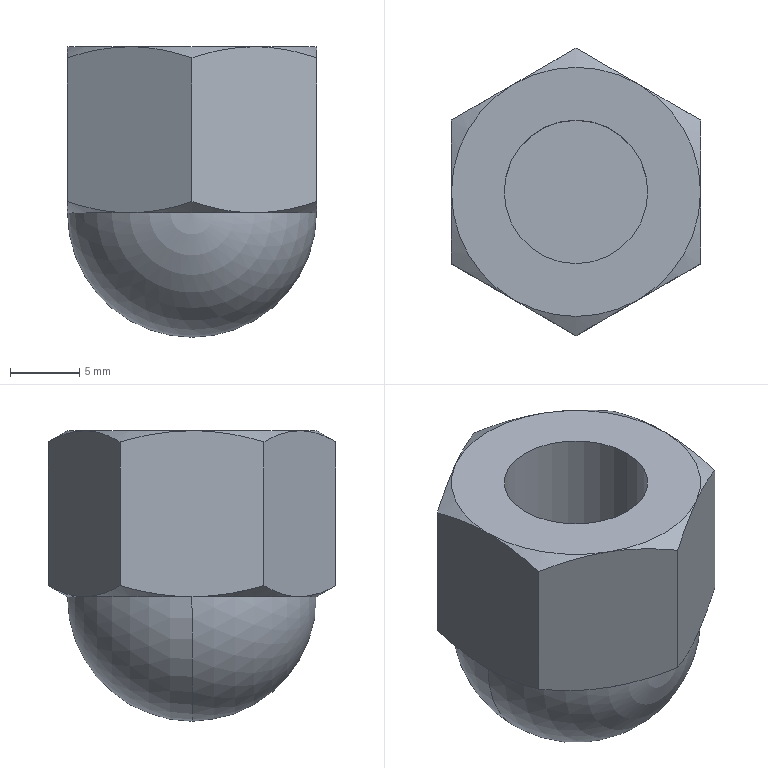Part | SolidWorks | features Cut 3, Extrusion 1, Revolution 1 | 1 solid | 24 faces | box 18 x 20.785 x 21 mm | volume 4036 mm3 | cone 12 | plane 8 | cylinder 2 | sphere 2 | commonest cylinder face diameters 10.376 x2
STEP:
#1=CARTESIAN_POINT('',(-5.188,0.,2.));
#2=VERTEX_POINT('',#1);
#3=CARTESIAN_POINT('',(5.188,0.,2.));
#4=VERTEX_POINT('',#3);
#5=CARTESIAN_POINT('',(0.,0.,2.));
#6=DIRECTION('',(0.,0.,1.));
#7=DIRECTION('',(1.,0.,0.));
#8=AXIS2_PLACEMENT_3D('',#5,#6,#7);
#9=CIRCLE('',#8,5.188);
#10=EDGE_CURVE('',#2,#4,#9,.T.);
#11=ORIENTED_EDGE('',*,*,#10,.F.);
#12=CARTESIAN_POINT('',(-5.188,0.,12.));
#13=VERTEX_POINT('',#12);
#14=CARTESIAN_POINT('',(-5.188,0.,2.));
#15=DIRECTION('',(0.,0.,1.));
#16=VECTOR('',#15,1000.);
#17=LINE('',#14,#16);
#18=EDGE_CURVE('',#2,#13,#17,.T.);
#19=ORIENTED_EDGE('',*,*,#18,.T.);
#20=CARTESIAN_POINT('',(5.188,0.,12.));
#21=VERTEX_POINT('',#20);
#22=CARTESIAN_POINT('',(0.,0.,12.));
#23=DIRECTION('',(0.,0.,1.));
#24=DIRECTION('',(1.,0.,0.));
#25=AXIS2_PLACEMENT_3D('',#22,#23,#24);
#26=CIRCLE('',#25,5.188);
#27=EDGE_CURVE('',#13,#21,#26,.T.);
#28=ORIENTED_EDGE('',*,*,#27,.T.);
#29=CARTESIAN_POINT('',(5.188,0.,2.));
#30=DIRECTION('',(0.,0.,1.));
#31=VECTOR('',#30,1000.);
#32=LINE('',#29,#31);
#33=EDGE_CURVE('',#4,#21,#32,.T.);
#34=ORIENTED_EDGE('',*,*,#33,.F.);
#35=EDGE_LOOP('',(#11,#19,#28,#34));
#36=FACE_OUTER_BOUND('',#35,.T.);
#37=CARTESIAN_POINT('',(0.,0.,2.));
#38=DIRECTION('',(0.,0.,1.));
#39=DIRECTION('',(1.,0.,0.));
#40=AXIS2_PLACEMENT_3D('',#37,#38,#39);
#41=CYLINDRICAL_SURFACE('',#40,5.188);
#42=ADVANCED_FACE('',(#36),#41,.F.);
#43=CARTESIAN_POINT('',(-9.,0.,0.));
#44=VERTEX_POINT('',#43);
#45=CARTESIAN_POINT('',(-4.5,-7.794,0.));
#46=VERTEX_POINT('',#45);
#47=CARTESIAN_POINT('',(0.,0.,0.));
#48=DIRECTION('',(0.,0.,1.));
#49=DIRECTION('',(-1.,0.,0.));
#50=AXIS2_PLACEMENT_3D('',#47,#48,#49);
#51=CIRCLE('',#50,9.);
#52=EDGE_CURVE('',#44,#46,#51,.T.);
#53=ORIENTED_EDGE('',*,*,#52,.F.);
#54=CARTESIAN_POINT('',(0.,0.,-9.));
#55=VERTEX_POINT('',#54);
#56=CARTESIAN_POINT('',(0.,0.,0.));
#57=DIRECTION('',(0.,-1.,0.));
#58=DIRECTION('',(1.,0.,0.));
#59=AXIS2_PLACEMENT_3D('',#56,#57,#58);
#60=CIRCLE('',#59,9.);
#61=EDGE_CURVE('',#44,#55,#60,.T.);
#62=ORIENTED_EDGE('',*,*,#61,.T.);
#63=CARTESIAN_POINT('',(9.,0.,0.));
#64=VERTEX_POINT('',#63);
#65=CARTESIAN_POINT('',(0.,0.,0.));
#66=DIRECTION('',(0.,1.,0.));
#67=DIRECTION('',(0.,0.,1.));
#68=AXIS2_PLACEMENT_3D('',#65,#66,#67);
#69=CIRCLE('',#68,9.);
#70=EDGE_CURVE('',#64,#55,#69,.T.);
#71=ORIENTED_EDGE('',*,*,#70,.F.);
#72=CARTESIAN_POINT('',(4.5,-7.794,0.));
#73=VERTEX_POINT('',#72);
#74=CARTESIAN_POINT('',(0.,0.,0.));
#75=DIRECTION('',(0.,0.,1.));
#76=DIRECTION('',(-1.,0.,0.));
#77=AXIS2_PLACEMENT_3D('',#74,#75,#76);
#78=CIRCLE('',#77,9.);
#79=EDGE_CURVE('',#73,#64,#78,.T.);
#80=ORIENTED_EDGE('',*,*,#79,.F.);
#81=CARTESIAN_POINT('',(0.,0.,0.));
#82=DIRECTION('',(0.,0.,1.));
#83=DIRECTION('',(-1.,0.,0.));
#84=AXIS2_PLACEMENT_3D('',#81,#82,#83);
#85=CIRCLE('',#84,9.);
#86=EDGE_CURVE('',#46,#73,#85,.T.);
#87=ORIENTED_EDGE('',*,*,#86,.F.);
#88=EDGE_LOOP('',(#53,#62,#71,#80,#87));
#89=FACE_OUTER_BOUND('',#88,.T.);
#90=CARTESIAN_POINT('',(0.,0.,0.));
#91=DIRECTION('',(0.,-1.,0.));
#92=DIRECTION('',(1.,0.,0.));
#93=AXIS2_PLACEMENT_3D('',#90,#91,#92);
#94=SPHERICAL_SURFACE('',#93,9.);
#95=ADVANCED_FACE('',(#89),#94,.T.);
#96=CARTESIAN_POINT('',(9.,5.196,11.196));
#97=VERTEX_POINT('',#96);
#98=CARTESIAN_POINT('',(4.5,7.794,12.));
#99=VERTEX_POINT('',#98);
#100=CARTESIAN_POINT('',(9.,5.196,11.196));
#101=CARTESIAN_POINT('',(8.264,5.621,11.442));
#102=CARTESIAN_POINT('',(7.522,6.049,11.644));
#103=CARTESIAN_POINT('',(6.024,6.914,11.923));
#104=CARTESIAN_POINT('',(5.267,7.352,12.));
#105=CARTESIAN_POINT('',(4.5,7.794,12.));
#106=B_SPLINE_CURVE_WITH_KNOTS('',3,(#100,#101,#102,#103,#104,#105),.UNSPECIFIED.,.F.,.F.,(4,2,4),(0.000000238,0.002629,0.005258),.UNSPECIFIED.);
#107=EDGE_CURVE('',#97,#99,#106,.T.);
#108=ORIENTED_EDGE('',*,*,#107,.F.);
#109=CARTESIAN_POINT('',(9.,5.196,0.8038));
#110=VERTEX_POINT('',#109);
#111=CARTESIAN_POINT('',(9.,5.196,12.));
#112=DIRECTION('',(0.,0.,-1.));
#113=VECTOR('',#112,1000.);
#114=LINE('',#111,#113);
#115=EDGE_CURVE('',#97,#110,#114,.T.);
#116=ORIENTED_EDGE('',*,*,#115,.T.);
#117=CARTESIAN_POINT('',(4.5,7.794,0.));
#118=VERTEX_POINT('',#117);
#119=CARTESIAN_POINT('',(4.5,7.794,0.));
#120=CARTESIAN_POINT('',(4.882,7.574,0.));
#121=CARTESIAN_POINT('',(5.266,7.352,0.019));
#122=CARTESIAN_POINT('',(6.024,6.914,0.09253));
#123=CARTESIAN_POINT('',(6.401,6.697,0.147));
#124=CARTESIAN_POINT('',(7.525,6.048,0.357));
#125=CARTESIAN_POINT('',(8.266,5.62,0.5591));
#126=CARTESIAN_POINT('',(9.,5.196,0.8038));
#127=B_SPLINE_CURVE_WITH_KNOTS('',3,(#119,#120,#121,#122,#123,#124,#125,#126),.UNSPECIFIED.,.F.,.F.,(4,2,2,4),(0.005258,0.006567,0.007877,0.0105),.UNSPECIFIED.);
#128=EDGE_CURVE('',#118,#110,#127,.T.);
#129=ORIENTED_EDGE('',*,*,#128,.F.);
#130=CARTESIAN_POINT('',(0.,10.392,0.8038));
#131=VERTEX_POINT('',#130);
#132=CARTESIAN_POINT('',(0.,10.392,0.8038));
#133=CARTESIAN_POINT('',(0.7361,9.967,0.5585));
#134=CARTESIAN_POINT('',(1.478,9.539,0.3563));
#135=CARTESIAN_POINT('',(2.976,8.674,0.07661));
#136=CARTESIAN_POINT('',(3.733,8.237,0.));
#137=CARTESIAN_POINT('',(4.5,7.794,0.));
#138=B_SPLINE_CURVE_WITH_KNOTS('',3,(#132,#133,#134,#135,#136,#137),.UNSPECIFIED.,.F.,.F.,(4,2,4),(0.000000238,0.002629,0.005258),.UNSPECIFIED.);
#139=EDGE_CURVE('',#131,#118,#138,.T.);
#140=ORIENTED_EDGE('',*,*,#139,.F.);
#141=CARTESIAN_POINT('',(0.,10.392,11.196));
#142=VERTEX_POINT('',#141);
#143=CARTESIAN_POINT('',(0.,10.392,12.));
#144=DIRECTION('',(0.,0.,-1.));
#145=VECTOR('',#144,1000.);
#146=LINE('',#143,#145);
#147=EDGE_CURVE('',#142,#131,#146,.T.);
#148=ORIENTED_EDGE('',*,*,#147,.F.);
#149=CARTESIAN_POINT('',(4.5,7.794,12.));
#150=CARTESIAN_POINT('',(4.118,8.015,12.));
#151=CARTESIAN_POINT('',(3.734,8.236,11.981));
#152=CARTESIAN_POINT('',(2.976,8.674,11.907));
#153=CARTESIAN_POINT('',(2.599,8.892,11.853));
#154=CARTESIAN_POINT('',(1.475,9.541,11.643));
#155=CARTESIAN_POINT('',(0.7343,9.968,11.441));
#156=CARTESIAN_POINT('',(0.,10.392,11.196));
#157=B_SPLINE_CURVE_WITH_KNOTS('',3,(#149,#150,#151,#152,#153,#154,#155,#156),.UNSPECIFIED.,.F.,.F.,(4,2,2,4),(0.005258,0.006567,0.007877,0.0105),.UNSPECIFIED.);
#158=EDGE_CURVE('',#99,#142,#157,.T.);
#159=ORIENTED_EDGE('',*,*,#158,.F.);
#160=EDGE_LOOP('',(#108,#116,#129,#140,#148,#159));
#161=FACE_OUTER_BOUND('',#160,.T.);
#162=CARTESIAN_POINT('',(9.,5.196,12.));
#163=DIRECTION('',(-0.5,-0.866,0.));
#164=DIRECTION('',(0.866,-0.5,0.));
#165=AXIS2_PLACEMENT_3D('',#162,#163,#164);
#166=PLANE('',#165);
#167=ADVANCED_FACE('',(#161),#166,.F.);
#168=CARTESIAN_POINT('',(-4.5,7.794,12.));
#169=VERTEX_POINT('',#168);
#170=CARTESIAN_POINT('',(0.,10.392,11.196));
#171=CARTESIAN_POINT('',(-0.7361,9.967,11.442));
#172=CARTESIAN_POINT('',(-1.478,9.539,11.644));
#173=CARTESIAN_POINT('',(-2.976,8.674,11.923));
#174=CARTESIAN_POINT('',(-3.733,8.237,12.));
#175=CARTESIAN_POINT('',(-4.5,7.794,12.));
#176=B_SPLINE_CURVE_WITH_KNOTS('',3,(#170,#171,#172,#173,#174,#175),.UNSPECIFIED.,.F.,.F.,(4,2,4),(0.000000238,0.002629,0.005258),.UNSPECIFIED.);
#177=EDGE_CURVE('',#142,#169,#176,.T.);
#178=ORIENTED_EDGE('',*,*,#177,.F.);
#179=ORIENTED_EDGE('',*,*,#147,.T.);
#180=CARTESIAN_POINT('',(-4.5,7.794,0.));
#181=VERTEX_POINT('',#180);
#182=CARTESIAN_POINT('',(-4.5,7.794,0.));
#183=CARTESIAN_POINT('',(-4.118,8.015,0.));
#184=CARTESIAN_POINT('',(-3.734,8.236,0.019));
#185=CARTESIAN_POINT('',(-2.976,8.674,0.09253));
#186=CARTESIAN_POINT('',(-2.599,8.892,0.147));
#187=CARTESIAN_POINT('',(-1.475,9.541,0.357));
#188=CARTESIAN_POINT('',(-0.7343,9.968,0.5591));
#189=CARTESIAN_POINT('',(0.,10.392,0.8038));
#190=B_SPLINE_CURVE_WITH_KNOTS('',3,(#182,#183,#184,#185,#186,#187,#188,#189),.UNSPECIFIED.,.F.,.F.,(4,2,2,4),(0.005258,0.006567,0.007877,0.0105),.UNSPECIFIED.);
#191=EDGE_CURVE('',#181,#131,#190,.T.);
#192=ORIENTED_EDGE('',*,*,#191,.F.);
#193=CARTESIAN_POINT('',(-9.,5.196,0.8038));
#194=VERTEX_POINT('',#193);
#195=CARTESIAN_POINT('',(-9.,5.196,0.8038));
#196=CARTESIAN_POINT('',(-8.264,5.621,0.5585));
#197=CARTESIAN_POINT('',(-7.522,6.049,0.3563));
#198=CARTESIAN_POINT('',(-6.024,6.914,0.07661));
#199=CARTESIAN_POINT('',(-5.267,7.352,0.));
#200=CARTESIAN_POINT('',(-4.5,7.794,0.));
#201=B_SPLINE_CURVE_WITH_KNOTS('',3,(#195,#196,#197,#198,#199,#200),.UNSPECIFIED.,.F.,.F.,(4,2,4),(0.000000238,0.002629,0.005258),.UNSPECIFIED.);
#202=EDGE_CURVE('',#194,#181,#201,.T.);
#203=ORIENTED_EDGE('',*,*,#202,.F.);
#204=CARTESIAN_POINT('',(-9.,5.196,11.196));
#205=VERTEX_POINT('',#204);
#206=CARTESIAN_POINT('',(-9.,5.196,12.));
#207=DIRECTION('',(0.,0.,-1.));
#208=VECTOR('',#207,1000.);
#209=LINE('',#206,#208);
#210=EDGE_CURVE('',#205,#194,#209,.T.);
#211=ORIENTED_EDGE('',*,*,#210,.F.);
#212=CARTESIAN_POINT('',(-4.5,7.794,12.));
#213=CARTESIAN_POINT('',(-4.882,7.574,12.));
#214=CARTESIAN_POINT('',(-5.266,7.352,11.981));
#215=CARTESIAN_POINT('',(-6.024,6.914,11.907));
#216=CARTESIAN_POINT('',(-6.401,6.697,11.853));
#217=CARTESIAN_POINT('',(-7.525,6.048,11.643));
#218=CARTESIAN_POINT('',(-8.266,5.62,11.441));
#219=CARTESIAN_POINT('',(-9.,5.196,11.196));
#220=B_SPLINE_CURVE_WITH_KNOTS('',3,(#212,#213,#214,#215,#216,#217,#218,#219),.UNSPECIFIED.,.F.,.F.,(4,2,2,4),(0.005258,0.006567,0.007877,0.0105),.UNSPECIFIED.);
#221=EDGE_CURVE('',#169,#205,#220,.T.);
#222=ORIENTED_EDGE('',*,*,#221,.F.);
#223=EDGE_LOOP('',(#178,#179,#192,#203,#211,#222));
#224=FACE_OUTER_BOUND('',#223,.T.);
#225=CARTESIAN_POINT('',(0.,10.392,12.));
#226=DIRECTION('',(0.5,-0.866,0.));
#227=DIRECTION('',(0.866,0.5,0.));
#228=AXIS2_PLACEMENT_3D('',#225,#226,#227);
#229=PLANE('',#228);
#230=ADVANCED_FACE('',(#224),#229,.F.);
#231=CARTESIAN_POINT('',(-9.,0.,12.));
#232=VERTEX_POINT('',#231);
#233=CARTESIAN_POINT('',(-9.,5.196,11.196));
#234=CARTESIAN_POINT('',(-9.,4.356,11.439));
#235=CARTESIAN_POINT('',(-9.,3.505,11.641));
#236=CARTESIAN_POINT('',(-9.,2.204,11.852));
#237=CARTESIAN_POINT('',(-9.,1.767,11.907));
#238=CARTESIAN_POINT('',(-9.,0.8823,11.981));
#239=CARTESIAN_POINT('',(-9.,0.4399,12.));
#240=CARTESIAN_POINT('',(-9.,0.,12.));
#241=B_SPLINE_CURVE_WITH_KNOTS('',3,(#233,#234,#235,#236,#237,#238,#239,#240),.UNSPECIFIED.,.F.,.F.,(4,2,2,4),(0.03305,0.03568,0.03699,0.0383),.UNSPECIFIED.);
#242=EDGE_CURVE('',#205,#232,#241,.T.);
#243=ORIENTED_EDGE('',*,*,#242,.F.);
#244=ORIENTED_EDGE('',*,*,#210,.T.);
#245=CARTESIAN_POINT('',(-9.,0.,0.));
#246=CARTESIAN_POINT('',(-9.,0.4398,0.));
#247=CARTESIAN_POINT('',(-9.,0.8817,0.01876));
#248=CARTESIAN_POINT('',(-9.,1.766,0.0931));
#249=CARTESIAN_POINT('',(-9.,2.204,0.1481));
#250=CARTESIAN_POINT('',(-9.,3.505,0.3593));
#251=CARTESIAN_POINT('',(-9.,4.356,0.5612));
#252=CARTESIAN_POINT('',(-9.,5.196,0.8038));
#253=B_SPLINE_CURVE_WITH_KNOTS('',3,(#245,#246,#247,#248,#249,#250,#251,#252),.UNSPECIFIED.,.F.,.F.,(4,2,2,4),(0.01481,0.01613,0.01744,0.02007),.UNSPECIFIED.);
#254=EDGE_CURVE('',#44,#194,#253,.T.);
#255=ORIENTED_EDGE('',*,*,#254,.F.);
#256=CARTESIAN_POINT('',(-9.,-5.196,0.8038));
#257=VERTEX_POINT('',#256);
#258=CARTESIAN_POINT('',(-9.,-5.196,0.8038));
#259=CARTESIAN_POINT('',(-9.,-4.35,0.5597));
#260=CARTESIAN_POINT('',(-9.,-3.485,0.3552));
#261=CARTESIAN_POINT('',(-9.,-1.751,0.0756));
#262=CARTESIAN_POINT('',(-9.,-0.8789,0.));
#263=CARTESIAN_POINT('',(-9.,0.,0.));
#264=B_SPLINE_CURVE_WITH_KNOTS('',3,(#258,#259,#260,#261,#262,#263),.UNSPECIFIED.,.F.,.F.,(4,2,4),(0.009551,0.01218,0.01481),.UNSPECIFIED.);
#265=EDGE_CURVE('',#257,#44,#264,.T.);
#266=ORIENTED_EDGE('',*,*,#265,.F.);
#267=CARTESIAN_POINT('',(-9.,-5.196,11.196));
#268=VERTEX_POINT('',#267);
#269=CARTESIAN_POINT('',(-9.,-5.196,12.));
#270=DIRECTION('',(0.,0.,-1.));
#271=VECTOR('',#270,1000.);
#272=LINE('',#269,#271);
#273=EDGE_CURVE('',#268,#257,#272,.T.);
#274=ORIENTED_EDGE('',*,*,#273,.F.);
#275=CARTESIAN_POINT('',(-9.,0.,12.));
#276=CARTESIAN_POINT('',(-9.,-0.8791,12.));
#277=CARTESIAN_POINT('',(-9.,-1.752,11.924));
#278=CARTESIAN_POINT('',(-9.,-3.485,11.645));
#279=CARTESIAN_POINT('',(-9.,-4.35,11.44));
#280=CARTESIAN_POINT('',(-9.,-5.196,11.196));
#281=B_SPLINE_CURVE_WITH_KNOTS('',3,(#275,#276,#277,#278,#279,#280),.UNSPECIFIED.,.F.,.F.,(4,2,4),(0.0383,0.04093,0.04356),.UNSPECIFIED.);
#282=EDGE_CURVE('',#232,#268,#281,.T.);
#283=ORIENTED_EDGE('',*,*,#282,.F.);
#284=EDGE_LOOP('',(#243,#244,#255,#266,#274,#283));
#285=FACE_OUTER_BOUND('',#284,.T.);
#286=CARTESIAN_POINT('',(-9.,5.196,12.));
#287=DIRECTION('',(1.,0.,0.));
#288=DIRECTION('',(0.,0.,-1.));
#289=AXIS2_PLACEMENT_3D('',#286,#287,#288);
#290=PLANE('',#289);
#291=ADVANCED_FACE('',(#285),#290,.F.);
#292=CARTESIAN_POINT('',(-4.5,-7.794,12.));
#293=VERTEX_POINT('',#292);
#294=CARTESIAN_POINT('',(-9.,-5.196,11.196));
#295=CARTESIAN_POINT('',(-8.264,-5.621,11.442));
#296=CARTESIAN_POINT('',(-7.522,-6.049,11.644));
#297=CARTESIAN_POINT('',(-6.024,-6.914,11.923));
#298=CARTESIAN_POINT('',(-5.267,-7.352,12.));
#299=CARTESIAN_POINT('',(-4.5,-7.794,12.));
#300=B_SPLINE_CURVE_WITH_KNOTS('',3,(#294,#295,#296,#297,#298,#299),.UNSPECIFIED.,.F.,.F.,(4,2,4),(0.000000238,0.002629,0.005258),.UNSPECIFIED.);
#301=EDGE_CURVE('',#268,#293,#300,.T.);
#302=ORIENTED_EDGE('',*,*,#301,.F.);
#303=ORIENTED_EDGE('',*,*,#273,.T.);
#304=CARTESIAN_POINT('',(-4.5,-7.794,0.));
#305=CARTESIAN_POINT('',(-4.882,-7.574,0.));
#306=CARTESIAN_POINT('',(-5.266,-7.352,0.019));
#307=CARTESIAN_POINT('',(-6.024,-6.914,0.09253));
#308=CARTESIAN_POINT('',(-6.401,-6.697,0.147));
#309=CARTESIAN_POINT('',(-7.525,-6.048,0.357));
#310=CARTESIAN_POINT('',(-8.266,-5.62,0.5591));
#311=CARTESIAN_POINT('',(-9.,-5.196,0.8038));
#312=B_SPLINE_CURVE_WITH_KNOTS('',3,(#304,#305,#306,#307,#308,#309,#310,#311),.UNSPECIFIED.,.F.,.F.,(4,2,2,4),(0.005258,0.006567,0.007877,0.0105),.UNSPECIFIED.);
#313=EDGE_CURVE('',#46,#257,#312,.T.);
#314=ORIENTED_EDGE('',*,*,#313,.F.);
#315=CARTESIAN_POINT('',(0.,-10.392,0.8038));
#316=VERTEX_POINT('',#315);
#317=CARTESIAN_POINT('',(0.,-10.392,0.8038));
#318=CARTESIAN_POINT('',(-0.7361,-9.967,0.5585));
#319=CARTESIAN_POINT('',(-1.478,-9.539,0.3563));
#320=CARTESIAN_POINT('',(-2.976,-8.674,0.07661));
#321=CARTESIAN_POINT('',(-3.733,-8.237,0.));
#322=CARTESIAN_POINT('',(-4.5,-7.794,0.));
#323=B_SPLINE_CURVE_WITH_KNOTS('',3,(#317,#318,#319,#320,#321,#322),.UNSPECIFIED.,.F.,.F.,(4,2,4),(0.000000238,0.002629,0.005258),.UNSPECIFIED.);
#324=EDGE_CURVE('',#316,#46,#323,.T.);
#325=ORIENTED_EDGE('',*,*,#324,.F.);
#326=CARTESIAN_POINT('',(0.,-10.392,11.196));
#327=VERTEX_POINT('',#326);
#328=CARTESIAN_POINT('',(0.,-10.392,12.));
#329=DIRECTION('',(0.,0.,-1.));
#330=VECTOR('',#329,1000.);
#331=LINE('',#328,#330);
#332=EDGE_CURVE('',#327,#316,#331,.T.);
#333=ORIENTED_EDGE('',*,*,#332,.F.);
#334=CARTESIAN_POINT('',(-4.5,-7.794,12.));
#335=CARTESIAN_POINT('',(-4.118,-8.015,12.));
#336=CARTESIAN_POINT('',(-3.734,-8.236,11.981));
#337=CARTESIAN_POINT('',(-2.976,-8.674,11.907));
#338=CARTESIAN_POINT('',(-2.599,-8.892,11.853));
#339=CARTESIAN_POINT('',(-1.475,-9.541,11.643));
#340=CARTESIAN_POINT('',(-0.7343,-9.968,11.441));
#341=CARTESIAN_POINT('',(0.,-10.392,11.196));
#342=B_SPLINE_CURVE_WITH_KNOTS('',3,(#334,#335,#336,#337,#338,#339,#340,#341),.UNSPECIFIED.,.F.,.F.,(4,2,2,4),(0.005258,0.006567,0.007877,0.0105),.UNSPECIFIED.);
#343=EDGE_CURVE('',#293,#327,#342,.T.);
#344=ORIENTED_EDGE('',*,*,#343,.F.);
#345=EDGE_LOOP('',(#302,#303,#314,#325,#333,#344));
#346=FACE_OUTER_BOUND('',#345,.T.);
#347=CARTESIAN_POINT('',(-9.,-5.196,12.));
#348=DIRECTION('',(0.5,0.866,0.));
#349=DIRECTION('',(-0.866,0.5,0.));
#350=AXIS2_PLACEMENT_3D('',#347,#348,#349);
#351=PLANE('',#350);
#352=ADVANCED_FACE('',(#346),#351,.F.);
#353=CARTESIAN_POINT('',(4.5,-7.794,12.));
#354=VERTEX_POINT('',#353);
#355=CARTESIAN_POINT('',(0.,-10.392,11.196));
#356=CARTESIAN_POINT('',(0.7361,-9.967,11.442));
#357=CARTESIAN_POINT('',(1.478,-9.539,11.644));
#358=CARTESIAN_POINT('',(2.976,-8.674,11.923));
#359=CARTESIAN_POINT('',(3.733,-8.237,12.));
#360=CARTESIAN_POINT('',(4.5,-7.794,12.));
#361=B_SPLINE_CURVE_WITH_KNOTS('',3,(#355,#356,#357,#358,#359,#360),.UNSPECIFIED.,.F.,.F.,(4,2,4),(0.000000238,0.002629,0.005258),.UNSPECIFIED.);
#362=EDGE_CURVE('',#327,#354,#361,.T.);
#363=ORIENTED_EDGE('',*,*,#362,.F.);
#364=ORIENTED_EDGE('',*,*,#332,.T.);
#365=CARTESIAN_POINT('',(4.5,-7.794,0.));
#366=CARTESIAN_POINT('',(4.118,-8.015,0.));
#367=CARTESIAN_POINT('',(3.734,-8.236,0.019));
#368=CARTESIAN_POINT('',(2.976,-8.674,0.09253));
#369=CARTESIAN_POINT('',(2.599,-8.892,0.147));
#370=CARTESIAN_POINT('',(1.475,-9.541,0.357));
#371=CARTESIAN_POINT('',(0.7343,-9.968,0.5591));
#372=CARTESIAN_POINT('',(0.,-10.392,0.8038));
#373=B_SPLINE_CURVE_WITH_KNOTS('',3,(#365,#366,#367,#368,#369,#370,#371,#372),.UNSPECIFIED.,.F.,.F.,(4,2,2,4),(0.005258,0.006567,0.007877,0.0105),.UNSPECIFIED.);
#374=EDGE_CURVE('',#73,#316,#373,.T.);
#375=ORIENTED_EDGE('',*,*,#374,.F.);
#376=CARTESIAN_POINT('',(9.,-5.196,0.8038));
#377=VERTEX_POINT('',#376);
#378=CARTESIAN_POINT('',(9.,-5.196,0.8038));
#379=CARTESIAN_POINT('',(8.264,-5.621,0.5585));
#380=CARTESIAN_POINT('',(7.522,-6.049,0.3563));
#381=CARTESIAN_POINT('',(6.024,-6.914,0.07661));
#382=CARTESIAN_POINT('',(5.267,-7.352,0.));
#383=CARTESIAN_POINT('',(4.5,-7.794,0.));
#384=B_SPLINE_CURVE_WITH_KNOTS('',3,(#378,#379,#380,#381,#382,#383),.UNSPECIFIED.,.F.,.F.,(4,2,4),(0.000000238,0.002629,0.005258),.UNSPECIFIED.);
#385=EDGE_CURVE('',#377,#73,#384,.T.);
#386=ORIENTED_EDGE('',*,*,#385,.F.);
#387=CARTESIAN_POINT('',(9.,-5.196,11.196));
#388=VERTEX_POINT('',#387);
#389=CARTESIAN_POINT('',(9.,-5.196,12.));
#390=DIRECTION('',(0.,0.,-1.));
#391=VECTOR('',#390,1000.);
#392=LINE('',#389,#391);
#393=EDGE_CURVE('',#388,#377,#392,.T.);
#394=ORIENTED_EDGE('',*,*,#393,.F.);
#395=CARTESIAN_POINT('',(4.5,-7.794,12.));
#396=CARTESIAN_POINT('',(4.882,-7.574,12.));
#397=CARTESIAN_POINT('',(5.266,-7.352,11.981));
#398=CARTESIAN_POINT('',(6.024,-6.914,11.907));
#399=CARTESIAN_POINT('',(6.401,-6.697,11.853));
#400=CARTESIAN_POINT('',(7.525,-6.048,11.643));
#401=CARTESIAN_POINT('',(8.266,-5.62,11.441));
#402=CARTESIAN_POINT('',(9.,-5.196,11.196));
#403=B_SPLINE_CURVE_WITH_KNOTS('',3,(#395,#396,#397,#398,#399,#400,#401,#402),.UNSPECIFIED.,.F.,.F.,(4,2,2,4),(0.005258,0.006567,0.007877,0.0105),.UNSPECIFIED.);
#404=EDGE_CURVE('',#354,#388,#403,.T.);
#405=ORIENTED_EDGE('',*,*,#404,.F.);
#406=EDGE_LOOP('',(#363,#364,#375,#386,#394,#405));
#407=FACE_OUTER_BOUND('',#406,.T.);
#408=CARTESIAN_POINT('',(0.,-10.392,12.));
#409=DIRECTION('',(-0.5,0.866,0.));
#410=DIRECTION('',(-0.866,-0.5,0.));
#411=AXIS2_PLACEMENT_3D('',#408,#409,#410);
#412=PLANE('',#411);
#413=ADVANCED_FACE('',(#407),#412,.F.);
#414=CARTESIAN_POINT('',(9.,0.,12.));
#415=VERTEX_POINT('',#414);
#416=CARTESIAN_POINT('',(9.,-5.196,11.196));
#417=CARTESIAN_POINT('',(9.,-4.35,11.44));
#418=CARTESIAN_POINT('',(9.,-3.485,11.645));
#419=CARTESIAN_POINT('',(9.,-1.752,11.924));
#420=CARTESIAN_POINT('',(9.,-0.8791,12.));
#421=CARTESIAN_POINT('',(9.,0.,12.));
#422=B_SPLINE_CURVE_WITH_KNOTS('',3,(#416,#417,#418,#419,#420,#421),.UNSPECIFIED.,.F.,.F.,(4,2,4),(0.009612,0.01224,0.01487),.UNSPECIFIED.);
#423=EDGE_CURVE('',#388,#415,#422,.T.);
#424=ORIENTED_EDGE('',*,*,#423,.F.);
#425=ORIENTED_EDGE('',*,*,#393,.T.);
#426=CARTESIAN_POINT('',(9.,0.,0.));
#427=CARTESIAN_POINT('',(9.,-0.8789,0.));
#428=CARTESIAN_POINT('',(9.,-1.751,0.0756));
#429=CARTESIAN_POINT('',(9.,-3.485,0.3552));
#430=CARTESIAN_POINT('',(9.,-4.35,0.5597));
#431=CARTESIAN_POINT('',(9.,-5.196,0.8038));
#432=B_SPLINE_CURVE_WITH_KNOTS('',3,(#426,#427,#428,#429,#430,#431),.UNSPECIFIED.,.F.,.F.,(4,2,4),(0.03549,0.03812,0.04075),.UNSPECIFIED.);
#433=EDGE_CURVE('',#64,#377,#432,.T.);
#434=ORIENTED_EDGE('',*,*,#433,.F.);
#435=CARTESIAN_POINT('',(9.,5.196,0.8038));
#436=CARTESIAN_POINT('',(9.,4.356,0.5612));
#437=CARTESIAN_POINT('',(9.,3.505,0.3593));
#438=CARTESIAN_POINT('',(9.,2.204,0.1481));
#439=CARTESIAN_POINT('',(9.,1.766,0.0931));
#440=CARTESIAN_POINT('',(9.,0.8817,0.01876));
#441=CARTESIAN_POINT('',(9.,0.4398,0.));
#442=CARTESIAN_POINT('',(9.,0.,0.));
#443=B_SPLINE_CURVE_WITH_KNOTS('',3,(#435,#436,#437,#438,#439,#440,#441,#442),.UNSPECIFIED.,.F.,.F.,(4,2,2,4),(0.03023,0.03286,0.03418,0.03549),.UNSPECIFIED.);
#444=EDGE_CURVE('',#110,#64,#443,.T.);
#445=ORIENTED_EDGE('',*,*,#444,.F.);
#446=ORIENTED_EDGE('',*,*,#115,.F.);
#447=CARTESIAN_POINT('',(9.,0.,12.));
#448=CARTESIAN_POINT('',(9.,0.4399,12.));
#449=CARTESIAN_POINT('',(9.,0.8823,11.981));
#450=CARTESIAN_POINT('',(9.,1.767,11.907));
#451=CARTESIAN_POINT('',(9.,2.204,11.852));
#452=CARTESIAN_POINT('',(9.,3.505,11.641));
#453=CARTESIAN_POINT('',(9.,4.356,11.439));
#454=CARTESIAN_POINT('',(9.,5.196,11.196));
#455=B_SPLINE_CURVE_WITH_KNOTS('',3,(#447,#448,#449,#450,#451,#452,#453,#454),.UNSPECIFIED.,.F.,.F.,(4,2,2,4),(0.01487,0.01619,0.0175,0.02014),.UNSPECIFIED.);
#456=EDGE_CURVE('',#415,#97,#455,.T.);
#457=ORIENTED_EDGE('',*,*,#456,.F.);
#458=EDGE_LOOP('',(#424,#425,#434,#445,#446,#457));
#459=FACE_OUTER_BOUND('',#458,.T.);
#460=CARTESIAN_POINT('',(9.,-5.196,12.));
#461=DIRECTION('',(-1.,0.,0.));
#462=DIRECTION('',(0.,-1.,0.));
#463=AXIS2_PLACEMENT_3D('',#460,#461,#462);
#464=PLANE('',#463);
#465=ADVANCED_FACE('',(#459),#464,.F.);
#466=ORIENTED_EDGE('',*,*,#265,.T.);
#467=ORIENTED_EDGE('',*,*,#52,.T.);
#468=ORIENTED_EDGE('',*,*,#313,.T.);
#469=EDGE_LOOP('',(#466,#467,#468));
#470=FACE_OUTER_BOUND('',#469,.T.);
#471=CARTESIAN_POINT('',(0.,0.,0.));
#472=DIRECTION('',(0.,0.,1.));
#473=DIRECTION('',(-1.,0.,0.));
#474=AXIS2_PLACEMENT_3D('',#471,#472,#473);
#475=CONICAL_SURFACE('',#474,9.,1.047);
#476=ADVANCED_FACE('',(#470),#475,.T.);
#477=ORIENTED_EDGE('',*,*,#324,.T.);
#478=ORIENTED_EDGE('',*,*,#86,.T.);
#479=ORIENTED_EDGE('',*,*,#374,.T.);
#480=EDGE_LOOP('',(#477,#478,#479));
#481=FACE_OUTER_BOUND('',#480,.T.);
#482=CARTESIAN_POINT('',(0.,0.,0.));
#483=DIRECTION('',(0.,0.,1.));
#484=DIRECTION('',(-1.,0.,0.));
#485=AXIS2_PLACEMENT_3D('',#482,#483,#484);
#486=CONICAL_SURFACE('',#485,9.,1.047);
#487=ADVANCED_FACE('',(#481),#486,.T.);
#488=ORIENTED_EDGE('',*,*,#385,.T.);
#489=ORIENTED_EDGE('',*,*,#79,.T.);
#490=ORIENTED_EDGE('',*,*,#433,.T.);
#491=EDGE_LOOP('',(#488,#489,#490));
#492=FACE_OUTER_BOUND('',#491,.T.);
#493=CARTESIAN_POINT('',(0.,0.,0.));
#494=DIRECTION('',(0.,0.,1.));
#495=DIRECTION('',(-1.,0.,0.));
#496=AXIS2_PLACEMENT_3D('',#493,#494,#495);
#497=CONICAL_SURFACE('',#496,9.,1.047);
#498=ADVANCED_FACE('',(#492),#497,.T.);
#499=ORIENTED_EDGE('',*,*,#128,.T.);
#500=ORIENTED_EDGE('',*,*,#444,.T.);
#501=CARTESIAN_POINT('',(0.,0.,0.));
#502=DIRECTION('',(0.,0.,1.));
#503=DIRECTION('',(-1.,0.,0.));
#504=AXIS2_PLACEMENT_3D('',#501,#502,#503);
#505=CIRCLE('',#504,9.);
#506=EDGE_CURVE('',#64,#118,#505,.T.);
#507=ORIENTED_EDGE('',*,*,#506,.T.);
#508=EDGE_LOOP('',(#499,#500,#507));
#509=FACE_OUTER_BOUND('',#508,.T.);
#510=CARTESIAN_POINT('',(0.,0.,0.));
#511=DIRECTION('',(0.,0.,1.));
#512=DIRECTION('',(-1.,0.,0.));
#513=AXIS2_PLACEMENT_3D('',#510,#511,#512);
#514=CONICAL_SURFACE('',#513,9.,1.047);
#515=ADVANCED_FACE('',(#509),#514,.T.);
#516=ORIENTED_EDGE('',*,*,#191,.T.);
#517=ORIENTED_EDGE('',*,*,#139,.T.);
#518=CARTESIAN_POINT('',(0.,0.,0.));
#519=DIRECTION('',(0.,0.,1.));
#520=DIRECTION('',(-1.,0.,0.));
#521=AXIS2_PLACEMENT_3D('',#518,#519,#520);
#522=CIRCLE('',#521,9.);
#523=EDGE_CURVE('',#118,#181,#522,.T.);
#524=ORIENTED_EDGE('',*,*,#523,.T.);
#525=EDGE_LOOP('',(#516,#517,#524));
#526=FACE_OUTER_BOUND('',#525,.T.);
#527=CARTESIAN_POINT('',(0.,0.,0.));
#528=DIRECTION('',(0.,0.,1.));
#529=DIRECTION('',(-1.,0.,0.));
#530=AXIS2_PLACEMENT_3D('',#527,#528,#529);
#531=CONICAL_SURFACE('',#530,9.,1.047);
#532=ADVANCED_FACE('',(#526),#531,.T.);
#533=ORIENTED_EDGE('',*,*,#254,.T.);
#534=ORIENTED_EDGE('',*,*,#202,.T.);
#535=CARTESIAN_POINT('',(0.,0.,0.));
#536=DIRECTION('',(0.,0.,-1.));
#537=DIRECTION('',(-1.,0.,0.));
#538=AXIS2_PLACEMENT_3D('',#535,#536,#537);
#539=CIRCLE('',#538,9.);
#540=EDGE_CURVE('',#44,#181,#539,.T.);
#541=ORIENTED_EDGE('',*,*,#540,.F.);
#542=EDGE_LOOP('',(#533,#534,#541));
#543=FACE_OUTER_BOUND('',#542,.T.);
#544=CARTESIAN_POINT('',(0.,0.,0.));
#545=DIRECTION('',(0.,0.,1.));
#546=DIRECTION('',(-1.,0.,0.));
#547=AXIS2_PLACEMENT_3D('',#544,#545,#546);
#548=CONICAL_SURFACE('',#547,9.,1.047);
#549=ADVANCED_FACE('',(#543),#548,.T.);
#550=ORIENTED_EDGE('',*,*,#61,.F.);
#551=ORIENTED_EDGE('',*,*,#540,.T.);
#552=ORIENTED_EDGE('',*,*,#523,.F.);
#553=ORIENTED_EDGE('',*,*,#506,.F.);
#554=ORIENTED_EDGE('',*,*,#70,.T.);
#555=EDGE_LOOP('',(#550,#551,#552,#553,#554));
#556=FACE_OUTER_BOUND('',#555,.T.);
#557=CARTESIAN_POINT('',(0.,0.,0.));
#558=DIRECTION('',(0.,-1.,0.));
#559=DIRECTION('',(1.,0.,0.));
#560=AXIS2_PLACEMENT_3D('',#557,#558,#559);
#561=SPHERICAL_SURFACE('',#560,9.);
#562=ADVANCED_FACE('',(#556),#561,.T.);
#563=ORIENTED_EDGE('',*,*,#282,.T.);
#564=ORIENTED_EDGE('',*,*,#301,.T.);
#565=CARTESIAN_POINT('',(0.,0.,12.));
#566=DIRECTION('',(0.,0.,-1.));
#567=DIRECTION('',(-1.,0.,0.));
#568=AXIS2_PLACEMENT_3D('',#565,#566,#567);
#569=CIRCLE('',#568,9.);
#570=EDGE_CURVE('',#293,#232,#569,.T.);
#571=ORIENTED_EDGE('',*,*,#570,.T.);
#572=EDGE_LOOP('',(#563,#564,#571));
#573=FACE_OUTER_BOUND('',#572,.T.);
#574=CARTESIAN_POINT('',(0.,0.,12.));
#575=DIRECTION('',(0.,0.,-1.));
#576=DIRECTION('',(1.,0.,0.));
#577=AXIS2_PLACEMENT_3D('',#574,#575,#576);
#578=CONICAL_SURFACE('',#577,9.,1.047);
#579=ADVANCED_FACE('',(#573),#578,.T.);
#580=ORIENTED_EDGE('',*,*,#343,.T.);
#581=ORIENTED_EDGE('',*,*,#362,.T.);
#582=CARTESIAN_POINT('',(0.,0.,12.));
#583=DIRECTION('',(0.,0.,-1.));
#584=DIRECTION('',(-1.,0.,0.));
#585=AXIS2_PLACEMENT_3D('',#582,#583,#584);
#586=CIRCLE('',#585,9.);
#587=EDGE_CURVE('',#354,#293,#586,.T.);
#588=ORIENTED_EDGE('',*,*,#587,.T.);
#589=EDGE_LOOP('',(#580,#581,#588));
#590=FACE_OUTER_BOUND('',#589,.T.);
#591=CARTESIAN_POINT('',(0.,0.,12.));
#592=DIRECTION('',(0.,0.,-1.));
#593=DIRECTION('',(1.,0.,0.));
#594=AXIS2_PLACEMENT_3D('',#591,#592,#593);
#595=CONICAL_SURFACE('',#594,9.,1.047);
#596=ADVANCED_FACE('',(#590),#595,.T.);
#597=ORIENTED_EDGE('',*,*,#404,.T.);
#598=ORIENTED_EDGE('',*,*,#423,.T.);
#599=CARTESIAN_POINT('',(0.,0.,12.));
#600=DIRECTION('',(0.,0.,-1.));
#601=DIRECTION('',(-1.,0.,0.));
#602=AXIS2_PLACEMENT_3D('',#599,#600,#601);
#603=CIRCLE('',#602,9.);
#604=EDGE_CURVE('',#415,#354,#603,.T.);
#605=ORIENTED_EDGE('',*,*,#604,.T.);
#606=EDGE_LOOP('',(#597,#598,#605));
#607=FACE_OUTER_BOUND('',#606,.T.);
#608=CARTESIAN_POINT('',(0.,0.,12.));
#609=DIRECTION('',(0.,0.,-1.));
#610=DIRECTION('',(1.,0.,0.));
#611=AXIS2_PLACEMENT_3D('',#608,#609,#610);
#612=CONICAL_SURFACE('',#611,9.,1.047);
#613=ADVANCED_FACE('',(#607),#612,.T.);
#614=ORIENTED_EDGE('',*,*,#107,.T.);
#615=CARTESIAN_POINT('',(0.,0.,12.));
#616=DIRECTION('',(0.,0.,1.));
#617=DIRECTION('',(1.,0.,0.));
#618=AXIS2_PLACEMENT_3D('',#615,#616,#617);
#619=CIRCLE('',#618,9.);
#620=EDGE_CURVE('',#415,#99,#619,.T.);
#621=ORIENTED_EDGE('',*,*,#620,.F.);
#622=ORIENTED_EDGE('',*,*,#456,.T.);
#623=EDGE_LOOP('',(#614,#621,#622));
#624=FACE_OUTER_BOUND('',#623,.T.);
#625=CARTESIAN_POINT('',(0.,0.,12.));
#626=DIRECTION('',(0.,0.,-1.));
#627=DIRECTION('',(1.,0.,0.));
#628=AXIS2_PLACEMENT_3D('',#625,#626,#627);
#629=CONICAL_SURFACE('',#628,9.,1.047);
#630=ADVANCED_FACE('',(#624),#629,.T.);
#631=ORIENTED_EDGE('',*,*,#158,.T.);
#632=ORIENTED_EDGE('',*,*,#177,.T.);
#633=CARTESIAN_POINT('',(0.,0.,12.));
#634=DIRECTION('',(0.,0.,-1.));
#635=DIRECTION('',(-1.,0.,0.));
#636=AXIS2_PLACEMENT_3D('',#633,#634,#635);
#637=CIRCLE('',#636,9.);
#638=EDGE_CURVE('',#169,#99,#637,.T.);
#639=ORIENTED_EDGE('',*,*,#638,.T.);
#640=EDGE_LOOP('',(#631,#632,#639));
#641=FACE_OUTER_BOUND('',#640,.T.);
#642=CARTESIAN_POINT('',(0.,0.,12.));
#643=DIRECTION('',(0.,0.,-1.));
#644=DIRECTION('',(1.,0.,0.));
#645=AXIS2_PLACEMENT_3D('',#642,#643,#644);
#646=CONICAL_SURFACE('',#645,9.,1.047);
#647=ADVANCED_FACE('',(#641),#646,.T.);
#648=ORIENTED_EDGE('',*,*,#221,.T.);
#649=ORIENTED_EDGE('',*,*,#242,.T.);
#650=CARTESIAN_POINT('',(0.,0.,12.));
#651=DIRECTION('',(0.,0.,-1.));
#652=DIRECTION('',(-1.,0.,0.));
#653=AXIS2_PLACEMENT_3D('',#650,#651,#652);
#654=CIRCLE('',#653,9.);
#655=EDGE_CURVE('',#232,#169,#654,.T.);
#656=ORIENTED_EDGE('',*,*,#655,.T.);
#657=EDGE_LOOP('',(#648,#649,#656));
#658=FACE_OUTER_BOUND('',#657,.T.);
#659=CARTESIAN_POINT('',(0.,0.,12.));
#660=DIRECTION('',(0.,0.,-1.));
#661=DIRECTION('',(1.,0.,0.));
#662=AXIS2_PLACEMENT_3D('',#659,#660,#661);
#663=CONICAL_SURFACE('',#662,9.,1.047);
#664=ADVANCED_FACE('',(#658),#663,.T.);
#665=CARTESIAN_POINT('',(0.,0.,12.));
#666=DIRECTION('',(0.,0.,1.));
#667=DIRECTION('',(1.,0.,0.));
#668=AXIS2_PLACEMENT_3D('',#665,#666,#667);
#669=CIRCLE('',#668,5.188);
#670=EDGE_CURVE('',#21,#13,#669,.T.);
#671=ORIENTED_EDGE('',*,*,#670,.F.);
#672=ORIENTED_EDGE('',*,*,#27,.F.);
#673=EDGE_LOOP('',(#671,#672));
#674=FACE_BOUND('',#673,.T.);
#675=ORIENTED_EDGE('',*,*,#655,.F.);
#676=ORIENTED_EDGE('',*,*,#570,.F.);
#677=ORIENTED_EDGE('',*,*,#587,.F.);
#678=ORIENTED_EDGE('',*,*,#604,.F.);
#679=ORIENTED_EDGE('',*,*,#620,.T.);
#680=ORIENTED_EDGE('',*,*,#638,.F.);
#681=EDGE_LOOP('',(#675,#676,#677,#678,#679,#680));
#682=FACE_OUTER_BOUND('',#681,.T.);
#683=CARTESIAN_POINT('',(9.,5.196,12.));
#684=DIRECTION('',(0.,0.,-1.));
#685=DIRECTION('',(-1.,0.,0.));
#686=AXIS2_PLACEMENT_3D('',#683,#684,#685);
#687=PLANE('',#686);
#688=ADVANCED_FACE('',(#674,#682),#687,.F.);
#689=ORIENTED_EDGE('',*,*,#18,.F.);
#690=CARTESIAN_POINT('',(0.,0.,2.));
#691=DIRECTION('',(0.,0.,1.));
#692=DIRECTION('',(1.,0.,0.));
#693=AXIS2_PLACEMENT_3D('',#690,#691,#692);
#694=CIRCLE('',#693,5.188);
#695=EDGE_CURVE('',#4,#2,#694,.T.);
#696=ORIENTED_EDGE('',*,*,#695,.F.);
#697=ORIENTED_EDGE('',*,*,#33,.T.);
#698=ORIENTED_EDGE('',*,*,#670,.T.);
#699=EDGE_LOOP('',(#689,#696,#697,#698));
#700=FACE_OUTER_BOUND('',#699,.T.);
#701=CARTESIAN_POINT('',(0.,0.,2.));
#702=DIRECTION('',(0.,0.,1.));
#703=DIRECTION('',(1.,0.,0.));
#704=AXIS2_PLACEMENT_3D('',#701,#702,#703);
#705=CYLINDRICAL_SURFACE('',#704,5.188);
#706=ADVANCED_FACE('',(#700),#705,.F.);
#707=ORIENTED_EDGE('',*,*,#695,.T.);
#708=ORIENTED_EDGE('',*,*,#10,.T.);
#709=EDGE_LOOP('',(#707,#708));
#710=FACE_OUTER_BOUND('',#709,.T.);
#711=CARTESIAN_POINT('',(0.,0.,2.));
#712=DIRECTION('',(0.,0.,1.));
#713=DIRECTION('',(1.,0.,0.));
#714=AXIS2_PLACEMENT_3D('',#711,#712,#713);
#715=PLANE('',#714);
#716=ADVANCED_FACE('',(#710),#715,.T.);
#717=CLOSED_SHELL('',(#42,#95,#167,#230,#291,#352,#413,#465,#476,#487,#498,#515,#532,#549,#562,#579,#596,#613,#630,#647,#664,#688,#706,#716));
#718=MANIFOLD_SOLID_BREP('',#717);
#719=CARTESIAN_POINT('',(0.,0.,0.));
#720=DIRECTION('',(0.,0.,1.));
#721=DIRECTION('',(1.,0.,0.));
#722=AXIS2_PLACEMENT_3D('',#719,#720,#721);
#723=(LENGTH_UNIT()NAMED_UNIT(*)SI_UNIT(.MILLI.,.METRE.));
#724=UNCERTAINTY_MEASURE_WITH_UNIT(LENGTH_MEASURE(0.00001),#723,'','');
#725=(NAMED_UNIT(*)PLANE_ANGLE_UNIT()SI_UNIT($,.RADIAN.));
#726=(NAMED_UNIT(*)SI_UNIT($,.STERADIAN.)SOLID_ANGLE_UNIT());
#727=(GEOMETRIC_REPRESENTATION_CONTEXT(3)GLOBAL_UNCERTAINTY_ASSIGNED_CONTEXT((#724))GLOBAL_UNIT_ASSIGNED_CONTEXT((#723,#725,#726))REPRESENTATION_CONTEXT('',''));
#728=ADVANCED_BREP_SHAPE_REPRESENTATION('',(#718,#722),#727);